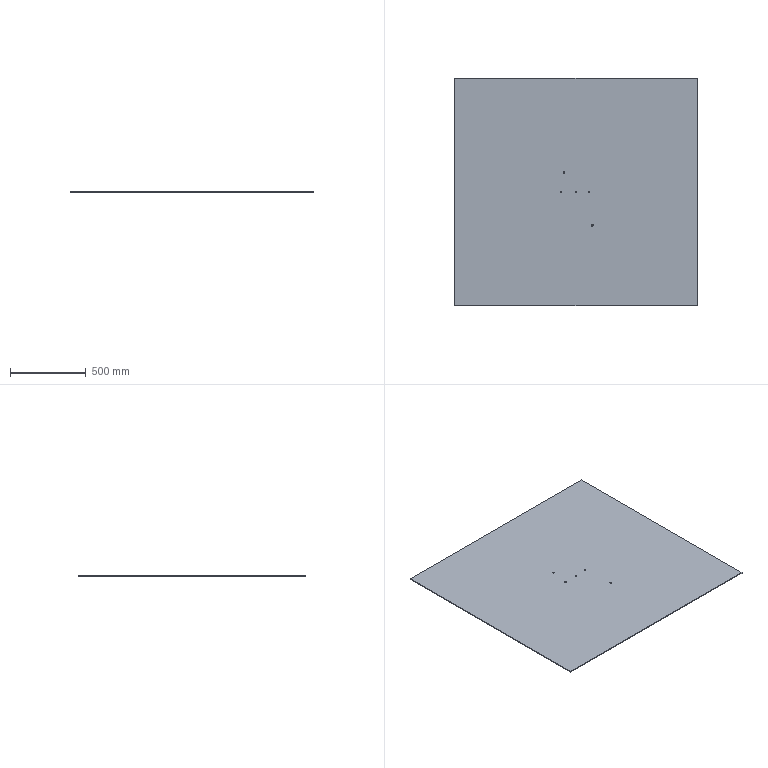Part | SolidWorks | features Extrusion 1 | 1 solid | 16 faces | box 1600 x 1500 x 5 mm | volume 11997688 mm3 | cylinder 10 | plane 6 | commonest cylinder face diameters 10 x6 10.014 x2 13.731 x2
STEP:
#1=CARTESIAN_POINT('',(-84.757,130.,5.));
#2=VERTEX_POINT('',#1);
#3=CARTESIAN_POINT('',(-74.743,130.,5.));
#4=VERTEX_POINT('',#3);
#5=CARTESIAN_POINT('',(-79.75,130.,5.));
#6=DIRECTION('',(0.,0.,1.));
#7=DIRECTION('',(1.,0.,0.));
#8=AXIS2_PLACEMENT_3D('',#5,#6,#7);
#9=CIRCLE('',#8,5.007);
#10=EDGE_CURVE('',#2,#4,#9,.T.);
#11=ORIENTED_EDGE('',*,*,#10,.T.);
#12=CARTESIAN_POINT('',(-74.743,130.,0.));
#13=VERTEX_POINT('',#12);
#14=CARTESIAN_POINT('',(-74.743,130.,5.));
#15=DIRECTION('',(0.,0.,-1.));
#16=VECTOR('',#15,1000.);
#17=LINE('',#14,#16);
#18=EDGE_CURVE('',#4,#13,#17,.T.);
#19=ORIENTED_EDGE('',*,*,#18,.T.);
#20=CARTESIAN_POINT('',(-84.757,130.,0.));
#21=VERTEX_POINT('',#20);
#22=CARTESIAN_POINT('',(-79.75,130.,0.));
#23=DIRECTION('',(0.,0.,1.));
#24=DIRECTION('',(1.,0.,0.));
#25=AXIS2_PLACEMENT_3D('',#22,#23,#24);
#26=CIRCLE('',#25,5.007);
#27=EDGE_CURVE('',#21,#13,#26,.T.);
#28=ORIENTED_EDGE('',*,*,#27,.F.);
#29=CARTESIAN_POINT('',(-84.757,130.,5.));
#30=DIRECTION('',(0.,0.,-1.));
#31=VECTOR('',#30,1000.);
#32=LINE('',#29,#31);
#33=EDGE_CURVE('',#2,#21,#32,.T.);
#34=ORIENTED_EDGE('',*,*,#33,.F.);
#35=EDGE_LOOP('',(#11,#19,#28,#34));
#36=FACE_OUTER_BOUND('',#35,.T.);
#37=CARTESIAN_POINT('',(-79.75,130.,5.));
#38=DIRECTION('',(0.,0.,-1.));
#39=DIRECTION('',(-1.,0.,0.));
#40=AXIS2_PLACEMENT_3D('',#37,#38,#39);
#41=CYLINDRICAL_SURFACE('',#40,5.007);
#42=ADVANCED_FACE('',(#36),#41,.F.);
#43=CARTESIAN_POINT('',(99.385,-219.089,5.));
#44=VERTEX_POINT('',#43);
#45=CARTESIAN_POINT('',(113.115,-219.089,5.));
#46=VERTEX_POINT('',#45);
#47=CARTESIAN_POINT('',(106.25,-219.089,5.));
#48=DIRECTION('',(0.,0.,1.));
#49=DIRECTION('',(1.,0.,0.));
#50=AXIS2_PLACEMENT_3D('',#47,#48,#49);
#51=CIRCLE('',#50,6.865);
#52=EDGE_CURVE('',#44,#46,#51,.T.);
#53=ORIENTED_EDGE('',*,*,#52,.T.);
#54=CARTESIAN_POINT('',(113.115,-219.089,0.));
#55=VERTEX_POINT('',#54);
#56=CARTESIAN_POINT('',(113.115,-219.089,5.));
#57=DIRECTION('',(0.,0.,-1.));
#58=VECTOR('',#57,1000.);
#59=LINE('',#56,#58);
#60=EDGE_CURVE('',#46,#55,#59,.T.);
#61=ORIENTED_EDGE('',*,*,#60,.T.);
#62=CARTESIAN_POINT('',(99.385,-219.089,0.));
#63=VERTEX_POINT('',#62);
#64=CARTESIAN_POINT('',(106.25,-219.089,0.));
#65=DIRECTION('',(0.,0.,1.));
#66=DIRECTION('',(1.,0.,0.));
#67=AXIS2_PLACEMENT_3D('',#64,#65,#66);
#68=CIRCLE('',#67,6.865);
#69=EDGE_CURVE('',#63,#55,#68,.T.);
#70=ORIENTED_EDGE('',*,*,#69,.F.);
#71=CARTESIAN_POINT('',(99.385,-219.089,5.));
#72=DIRECTION('',(0.,0.,-1.));
#73=VECTOR('',#72,1000.);
#74=LINE('',#71,#73);
#75=EDGE_CURVE('',#44,#63,#74,.T.);
#76=ORIENTED_EDGE('',*,*,#75,.F.);
#77=EDGE_LOOP('',(#53,#61,#70,#76));
#78=FACE_OUTER_BOUND('',#77,.T.);
#79=CARTESIAN_POINT('',(106.25,-219.089,5.));
#80=DIRECTION('',(0.,0.,-1.));
#81=DIRECTION('',(-1.,0.,0.));
#82=AXIS2_PLACEMENT_3D('',#79,#80,#81);
#83=CYLINDRICAL_SURFACE('',#82,6.865);
#84=ADVANCED_FACE('',(#78),#83,.F.);
#85=CARTESIAN_POINT('',(81.25,0.,5.));
#86=VERTEX_POINT('',#85);
#87=CARTESIAN_POINT('',(91.25,0.,5.));
#88=VERTEX_POINT('',#87);
#89=CARTESIAN_POINT('',(86.25,0.,5.));
#90=DIRECTION('',(0.,0.,1.));
#91=DIRECTION('',(1.,0.,0.));
#92=AXIS2_PLACEMENT_3D('',#89,#90,#91);
#93=CIRCLE('',#92,5.);
#94=EDGE_CURVE('',#86,#88,#93,.T.);
#95=ORIENTED_EDGE('',*,*,#94,.T.);
#96=CARTESIAN_POINT('',(91.25,0.,0.));
#97=VERTEX_POINT('',#96);
#98=CARTESIAN_POINT('',(91.25,0.,5.));
#99=DIRECTION('',(0.,0.,-1.));
#100=VECTOR('',#99,1000.);
#101=LINE('',#98,#100);
#102=EDGE_CURVE('',#88,#97,#101,.T.);
#103=ORIENTED_EDGE('',*,*,#102,.T.);
#104=CARTESIAN_POINT('',(81.25,0.,0.));
#105=VERTEX_POINT('',#104);
#106=CARTESIAN_POINT('',(86.25,0.,0.));
#107=DIRECTION('',(0.,0.,1.));
#108=DIRECTION('',(1.,0.,0.));
#109=AXIS2_PLACEMENT_3D('',#106,#107,#108);
#110=CIRCLE('',#109,5.);
#111=EDGE_CURVE('',#105,#97,#110,.T.);
#112=ORIENTED_EDGE('',*,*,#111,.F.);
#113=CARTESIAN_POINT('',(81.25,0.,5.));
#114=DIRECTION('',(0.,0.,-1.));
#115=VECTOR('',#114,1000.);
#116=LINE('',#113,#115);
#117=EDGE_CURVE('',#86,#105,#116,.T.);
#118=ORIENTED_EDGE('',*,*,#117,.F.);
#119=EDGE_LOOP('',(#95,#103,#112,#118));
#120=FACE_OUTER_BOUND('',#119,.T.);
#121=CARTESIAN_POINT('',(86.25,0.,5.));
#122=DIRECTION('',(0.,0.,-1.));
#123=DIRECTION('',(-1.,0.,0.));
#124=AXIS2_PLACEMENT_3D('',#121,#122,#123);
#125=CYLINDRICAL_SURFACE('',#124,5.);
#126=ADVANCED_FACE('',(#120),#125,.F.);
#127=CARTESIAN_POINT('',(-104.75,0.,5.));
#128=VERTEX_POINT('',#127);
#129=CARTESIAN_POINT('',(-94.75,0.,5.));
#130=VERTEX_POINT('',#129);
#131=CARTESIAN_POINT('',(-99.75,0.,5.));
#132=DIRECTION('',(0.,0.,1.));
#133=DIRECTION('',(1.,0.,0.));
#134=AXIS2_PLACEMENT_3D('',#131,#132,#133);
#135=CIRCLE('',#134,5.);
#136=EDGE_CURVE('',#128,#130,#135,.T.);
#137=ORIENTED_EDGE('',*,*,#136,.T.);
#138=CARTESIAN_POINT('',(-94.75,0.,0.));
#139=VERTEX_POINT('',#138);
#140=CARTESIAN_POINT('',(-94.75,0.,5.));
#141=DIRECTION('',(0.,0.,-1.));
#142=VECTOR('',#141,1000.);
#143=LINE('',#140,#142);
#144=EDGE_CURVE('',#130,#139,#143,.T.);
#145=ORIENTED_EDGE('',*,*,#144,.T.);
#146=CARTESIAN_POINT('',(-104.75,0.,0.));
#147=VERTEX_POINT('',#146);
#148=CARTESIAN_POINT('',(-99.75,0.,0.));
#149=DIRECTION('',(0.,0.,1.));
#150=DIRECTION('',(1.,0.,0.));
#151=AXIS2_PLACEMENT_3D('',#148,#149,#150);
#152=CIRCLE('',#151,5.);
#153=EDGE_CURVE('',#147,#139,#152,.T.);
#154=ORIENTED_EDGE('',*,*,#153,.F.);
#155=CARTESIAN_POINT('',(-104.75,0.,5.));
#156=DIRECTION('',(0.,0.,-1.));
#157=VECTOR('',#156,1000.);
#158=LINE('',#155,#157);
#159=EDGE_CURVE('',#128,#147,#158,.T.);
#160=ORIENTED_EDGE('',*,*,#159,.F.);
#161=EDGE_LOOP('',(#137,#145,#154,#160));
#162=FACE_OUTER_BOUND('',#161,.T.);
#163=CARTESIAN_POINT('',(-99.75,0.,5.));
#164=DIRECTION('',(0.,0.,-1.));
#165=DIRECTION('',(-1.,0.,0.));
#166=AXIS2_PLACEMENT_3D('',#163,#164,#165);
#167=CYLINDRICAL_SURFACE('',#166,5.);
#168=ADVANCED_FACE('',(#162),#167,.F.);
#169=CARTESIAN_POINT('',(-5.,0.,5.));
#170=VERTEX_POINT('',#169);
#171=CARTESIAN_POINT('',(5.,0.,5.));
#172=VERTEX_POINT('',#171);
#173=CARTESIAN_POINT('',(0.,0.,5.));
#174=DIRECTION('',(0.,0.,1.));
#175=DIRECTION('',(1.,0.,0.));
#176=AXIS2_PLACEMENT_3D('',#173,#174,#175);
#177=CIRCLE('',#176,5.);
#178=EDGE_CURVE('',#170,#172,#177,.T.);
#179=ORIENTED_EDGE('',*,*,#178,.T.);
#180=CARTESIAN_POINT('',(5.,0.,0.));
#181=VERTEX_POINT('',#180);
#182=CARTESIAN_POINT('',(5.,0.,5.));
#183=DIRECTION('',(0.,0.,-1.));
#184=VECTOR('',#183,1000.);
#185=LINE('',#182,#184);
#186=EDGE_CURVE('',#172,#181,#185,.T.);
#187=ORIENTED_EDGE('',*,*,#186,.T.);
#188=CARTESIAN_POINT('',(-5.,0.,0.));
#189=VERTEX_POINT('',#188);
#190=CARTESIAN_POINT('',(0.,0.,0.));
#191=DIRECTION('',(0.,0.,1.));
#192=DIRECTION('',(1.,0.,0.));
#193=AXIS2_PLACEMENT_3D('',#190,#191,#192);
#194=CIRCLE('',#193,5.);
#195=EDGE_CURVE('',#189,#181,#194,.T.);
#196=ORIENTED_EDGE('',*,*,#195,.F.);
#197=CARTESIAN_POINT('',(-5.,0.,5.));
#198=DIRECTION('',(0.,0.,-1.));
#199=VECTOR('',#198,1000.);
#200=LINE('',#197,#199);
#201=EDGE_CURVE('',#170,#189,#200,.T.);
#202=ORIENTED_EDGE('',*,*,#201,.F.);
#203=EDGE_LOOP('',(#179,#187,#196,#202));
#204=FACE_OUTER_BOUND('',#203,.T.);
#205=CARTESIAN_POINT('',(0.,0.,5.));
#206=DIRECTION('',(0.,0.,-1.));
#207=DIRECTION('',(-1.,0.,0.));
#208=AXIS2_PLACEMENT_3D('',#205,#206,#207);
#209=CYLINDRICAL_SURFACE('',#208,5.);
#210=ADVANCED_FACE('',(#204),#209,.F.);
#211=ORIENTED_EDGE('',*,*,#52,.F.);
#212=CARTESIAN_POINT('',(106.25,-219.089,5.));
#213=DIRECTION('',(0.,0.,1.));
#214=DIRECTION('',(1.,0.,0.));
#215=AXIS2_PLACEMENT_3D('',#212,#213,#214);
#216=CIRCLE('',#215,6.865);
#217=EDGE_CURVE('',#46,#44,#216,.T.);
#218=ORIENTED_EDGE('',*,*,#217,.F.);
#219=EDGE_LOOP('',(#211,#218));
#220=FACE_BOUND('',#219,.T.);
#221=ORIENTED_EDGE('',*,*,#136,.F.);
#222=CARTESIAN_POINT('',(-99.75,0.,5.));
#223=DIRECTION('',(0.,0.,1.));
#224=DIRECTION('',(1.,0.,0.));
#225=AXIS2_PLACEMENT_3D('',#222,#223,#224);
#226=CIRCLE('',#225,5.);
#227=EDGE_CURVE('',#130,#128,#226,.T.);
#228=ORIENTED_EDGE('',*,*,#227,.F.);
#229=EDGE_LOOP('',(#221,#228));
#230=FACE_BOUND('',#229,.T.);
#231=CARTESIAN_POINT('',(800.,-750.,5.));
#232=VERTEX_POINT('',#231);
#233=CARTESIAN_POINT('',(800.,750.,5.));
#234=VERTEX_POINT('',#233);
#235=CARTESIAN_POINT('',(800.,750.,5.));
#236=DIRECTION('',(0.,1.,0.));
#237=VECTOR('',#236,1000.);
#238=LINE('',#235,#237);
#239=EDGE_CURVE('',#232,#234,#238,.T.);
#240=ORIENTED_EDGE('',*,*,#239,.T.);
#241=CARTESIAN_POINT('',(-800.,750.,5.));
#242=VERTEX_POINT('',#241);
#243=CARTESIAN_POINT('',(-800.,750.,5.));
#244=DIRECTION('',(-1.,0.,0.));
#245=VECTOR('',#244,1000.);
#246=LINE('',#243,#245);
#247=EDGE_CURVE('',#234,#242,#246,.T.);
#248=ORIENTED_EDGE('',*,*,#247,.T.);
#249=CARTESIAN_POINT('',(-800.,-750.,5.));
#250=VERTEX_POINT('',#249);
#251=CARTESIAN_POINT('',(-800.,750.,5.));
#252=DIRECTION('',(0.,-1.,0.));
#253=VECTOR('',#252,1000.);
#254=LINE('',#251,#253);
#255=EDGE_CURVE('',#242,#250,#254,.T.);
#256=ORIENTED_EDGE('',*,*,#255,.T.);
#257=CARTESIAN_POINT('',(-800.,-750.,5.));
#258=DIRECTION('',(1.,0.,0.));
#259=VECTOR('',#258,1000.);
#260=LINE('',#257,#259);
#261=EDGE_CURVE('',#250,#232,#260,.T.);
#262=ORIENTED_EDGE('',*,*,#261,.T.);
#263=EDGE_LOOP('',(#240,#248,#256,#262));
#264=FACE_OUTER_BOUND('',#263,.T.);
#265=ORIENTED_EDGE('',*,*,#178,.F.);
#266=CARTESIAN_POINT('',(0.,0.,5.));
#267=DIRECTION('',(0.,0.,1.));
#268=DIRECTION('',(1.,0.,0.));
#269=AXIS2_PLACEMENT_3D('',#266,#267,#268);
#270=CIRCLE('',#269,5.);
#271=EDGE_CURVE('',#172,#170,#270,.T.);
#272=ORIENTED_EDGE('',*,*,#271,.F.);
#273=EDGE_LOOP('',(#265,#272));
#274=FACE_BOUND('',#273,.T.);
#275=ORIENTED_EDGE('',*,*,#94,.F.);
#276=CARTESIAN_POINT('',(86.25,0.,5.));
#277=DIRECTION('',(0.,0.,1.));
#278=DIRECTION('',(1.,0.,0.));
#279=AXIS2_PLACEMENT_3D('',#276,#277,#278);
#280=CIRCLE('',#279,5.);
#281=EDGE_CURVE('',#88,#86,#280,.T.);
#282=ORIENTED_EDGE('',*,*,#281,.F.);
#283=EDGE_LOOP('',(#275,#282));
#284=FACE_BOUND('',#283,.T.);
#285=ORIENTED_EDGE('',*,*,#10,.F.);
#286=CARTESIAN_POINT('',(-79.75,130.,5.));
#287=DIRECTION('',(0.,0.,1.));
#288=DIRECTION('',(1.,0.,0.));
#289=AXIS2_PLACEMENT_3D('',#286,#287,#288);
#290=CIRCLE('',#289,5.007);
#291=EDGE_CURVE('',#4,#2,#290,.T.);
#292=ORIENTED_EDGE('',*,*,#291,.F.);
#293=EDGE_LOOP('',(#285,#292));
#294=FACE_BOUND('',#293,.T.);
#295=CARTESIAN_POINT('',(0.,0.,5.));
#296=DIRECTION('',(0.,0.,1.));
#297=DIRECTION('',(1.,0.,0.));
#298=AXIS2_PLACEMENT_3D('',#295,#296,#297);
#299=PLANE('',#298);
#300=ADVANCED_FACE('',(#220,#230,#264,#274,#284,#294),#299,.T.);
#301=CARTESIAN_POINT('',(800.,-750.,0.));
#302=VERTEX_POINT('',#301);
#303=CARTESIAN_POINT('',(800.,750.,0.));
#304=VERTEX_POINT('',#303);
#305=CARTESIAN_POINT('',(800.,750.,0.));
#306=DIRECTION('',(0.,1.,0.));
#307=VECTOR('',#306,1000.);
#308=LINE('',#305,#307);
#309=EDGE_CURVE('',#302,#304,#308,.T.);
#310=ORIENTED_EDGE('',*,*,#309,.F.);
#311=CARTESIAN_POINT('',(-800.,-750.,0.));
#312=VERTEX_POINT('',#311);
#313=CARTESIAN_POINT('',(-800.,-750.,0.));
#314=DIRECTION('',(1.,0.,0.));
#315=VECTOR('',#314,1000.);
#316=LINE('',#313,#315);
#317=EDGE_CURVE('',#312,#302,#316,.T.);
#318=ORIENTED_EDGE('',*,*,#317,.F.);
#319=CARTESIAN_POINT('',(-800.,750.,0.));
#320=VERTEX_POINT('',#319);
#321=CARTESIAN_POINT('',(-800.,750.,0.));
#322=DIRECTION('',(0.,-1.,0.));
#323=VECTOR('',#322,1000.);
#324=LINE('',#321,#323);
#325=EDGE_CURVE('',#320,#312,#324,.T.);
#326=ORIENTED_EDGE('',*,*,#325,.F.);
#327=CARTESIAN_POINT('',(-800.,750.,0.));
#328=DIRECTION('',(-1.,0.,0.));
#329=VECTOR('',#328,1000.);
#330=LINE('',#327,#329);
#331=EDGE_CURVE('',#304,#320,#330,.T.);
#332=ORIENTED_EDGE('',*,*,#331,.F.);
#333=EDGE_LOOP('',(#310,#318,#326,#332));
#334=FACE_OUTER_BOUND('',#333,.T.);
#335=ORIENTED_EDGE('',*,*,#195,.T.);
#336=CARTESIAN_POINT('',(0.,0.,0.));
#337=DIRECTION('',(0.,0.,1.));
#338=DIRECTION('',(1.,0.,0.));
#339=AXIS2_PLACEMENT_3D('',#336,#337,#338);
#340=CIRCLE('',#339,5.);
#341=EDGE_CURVE('',#181,#189,#340,.T.);
#342=ORIENTED_EDGE('',*,*,#341,.T.);
#343=EDGE_LOOP('',(#335,#342));
#344=FACE_BOUND('',#343,.T.);
#345=ORIENTED_EDGE('',*,*,#153,.T.);
#346=CARTESIAN_POINT('',(-99.75,0.,0.));
#347=DIRECTION('',(0.,0.,1.));
#348=DIRECTION('',(1.,0.,0.));
#349=AXIS2_PLACEMENT_3D('',#346,#347,#348);
#350=CIRCLE('',#349,5.);
#351=EDGE_CURVE('',#139,#147,#350,.T.);
#352=ORIENTED_EDGE('',*,*,#351,.T.);
#353=EDGE_LOOP('',(#345,#352));
#354=FACE_BOUND('',#353,.T.);
#355=ORIENTED_EDGE('',*,*,#111,.T.);
#356=CARTESIAN_POINT('',(86.25,0.,0.));
#357=DIRECTION('',(0.,0.,1.));
#358=DIRECTION('',(1.,0.,0.));
#359=AXIS2_PLACEMENT_3D('',#356,#357,#358);
#360=CIRCLE('',#359,5.);
#361=EDGE_CURVE('',#97,#105,#360,.T.);
#362=ORIENTED_EDGE('',*,*,#361,.T.);
#363=EDGE_LOOP('',(#355,#362));
#364=FACE_BOUND('',#363,.T.);
#365=ORIENTED_EDGE('',*,*,#69,.T.);
#366=CARTESIAN_POINT('',(106.25,-219.089,0.));
#367=DIRECTION('',(0.,0.,1.));
#368=DIRECTION('',(1.,0.,0.));
#369=AXIS2_PLACEMENT_3D('',#366,#367,#368);
#370=CIRCLE('',#369,6.865);
#371=EDGE_CURVE('',#55,#63,#370,.T.);
#372=ORIENTED_EDGE('',*,*,#371,.T.);
#373=EDGE_LOOP('',(#365,#372));
#374=FACE_BOUND('',#373,.T.);
#375=ORIENTED_EDGE('',*,*,#27,.T.);
#376=CARTESIAN_POINT('',(-79.75,130.,0.));
#377=DIRECTION('',(0.,0.,1.));
#378=DIRECTION('',(1.,0.,0.));
#379=AXIS2_PLACEMENT_3D('',#376,#377,#378);
#380=CIRCLE('',#379,5.007);
#381=EDGE_CURVE('',#13,#21,#380,.T.);
#382=ORIENTED_EDGE('',*,*,#381,.T.);
#383=EDGE_LOOP('',(#375,#382));
#384=FACE_BOUND('',#383,.T.);
#385=CARTESIAN_POINT('',(0.,0.,0.));
#386=DIRECTION('',(0.,0.,1.));
#387=DIRECTION('',(1.,0.,0.));
#388=AXIS2_PLACEMENT_3D('',#385,#386,#387);
#389=PLANE('',#388);
#390=ADVANCED_FACE('',(#334,#344,#354,#364,#374,#384),#389,.F.);
#391=ORIENTED_EDGE('',*,*,#309,.T.);
#392=CARTESIAN_POINT('',(800.,750.,5.));
#393=DIRECTION('',(0.,0.,-1.));
#394=VECTOR('',#393,1000.);
#395=LINE('',#392,#394);
#396=EDGE_CURVE('',#234,#304,#395,.T.);
#397=ORIENTED_EDGE('',*,*,#396,.F.);
#398=ORIENTED_EDGE('',*,*,#239,.F.);
#399=CARTESIAN_POINT('',(800.,-750.,5.));
#400=DIRECTION('',(0.,0.,-1.));
#401=VECTOR('',#400,1000.);
#402=LINE('',#399,#401);
#403=EDGE_CURVE('',#232,#302,#402,.T.);
#404=ORIENTED_EDGE('',*,*,#403,.T.);
#405=EDGE_LOOP('',(#391,#397,#398,#404));
#406=FACE_OUTER_BOUND('',#405,.T.);
#407=CARTESIAN_POINT('',(800.,750.,5.));
#408=DIRECTION('',(-1.,0.,0.));
#409=DIRECTION('',(0.,0.,1.));
#410=AXIS2_PLACEMENT_3D('',#407,#408,#409);
#411=PLANE('',#410);
#412=ADVANCED_FACE('',(#406),#411,.F.);
#413=ORIENTED_EDGE('',*,*,#331,.T.);
#414=CARTESIAN_POINT('',(-800.,750.,5.));
#415=DIRECTION('',(0.,0.,-1.));
#416=VECTOR('',#415,1000.);
#417=LINE('',#414,#416);
#418=EDGE_CURVE('',#242,#320,#417,.T.);
#419=ORIENTED_EDGE('',*,*,#418,.F.);
#420=ORIENTED_EDGE('',*,*,#247,.F.);
#421=ORIENTED_EDGE('',*,*,#396,.T.);
#422=EDGE_LOOP('',(#413,#419,#420,#421));
#423=FACE_OUTER_BOUND('',#422,.T.);
#424=CARTESIAN_POINT('',(-800.,750.,5.));
#425=DIRECTION('',(0.,-1.,0.));
#426=DIRECTION('',(0.,0.,-1.));
#427=AXIS2_PLACEMENT_3D('',#424,#425,#426);
#428=PLANE('',#427);
#429=ADVANCED_FACE('',(#423),#428,.F.);
#430=ORIENTED_EDGE('',*,*,#325,.T.);
#431=CARTESIAN_POINT('',(-800.,-750.,5.));
#432=DIRECTION('',(0.,0.,-1.));
#433=VECTOR('',#432,1000.);
#434=LINE('',#431,#433);
#435=EDGE_CURVE('',#250,#312,#434,.T.);
#436=ORIENTED_EDGE('',*,*,#435,.F.);
#437=ORIENTED_EDGE('',*,*,#255,.F.);
#438=ORIENTED_EDGE('',*,*,#418,.T.);
#439=EDGE_LOOP('',(#430,#436,#437,#438));
#440=FACE_OUTER_BOUND('',#439,.T.);
#441=CARTESIAN_POINT('',(-800.,750.,5.));
#442=DIRECTION('',(1.,0.,0.));
#443=DIRECTION('',(0.,1.,0.));
#444=AXIS2_PLACEMENT_3D('',#441,#442,#443);
#445=PLANE('',#444);
#446=ADVANCED_FACE('',(#440),#445,.F.);
#447=ORIENTED_EDGE('',*,*,#317,.T.);
#448=ORIENTED_EDGE('',*,*,#403,.F.);
#449=ORIENTED_EDGE('',*,*,#261,.F.);
#450=ORIENTED_EDGE('',*,*,#435,.T.);
#451=EDGE_LOOP('',(#447,#448,#449,#450));
#452=FACE_OUTER_BOUND('',#451,.T.);
#453=CARTESIAN_POINT('',(-800.,-750.,5.));
#454=DIRECTION('',(0.,1.,0.));
#455=DIRECTION('',(-1.,0.,0.));
#456=AXIS2_PLACEMENT_3D('',#453,#454,#455);
#457=PLANE('',#456);
#458=ADVANCED_FACE('',(#452),#457,.F.);
#459=ORIENTED_EDGE('',*,*,#186,.F.);
#460=ORIENTED_EDGE('',*,*,#271,.T.);
#461=ORIENTED_EDGE('',*,*,#201,.T.);
#462=ORIENTED_EDGE('',*,*,#341,.F.);
#463=EDGE_LOOP('',(#459,#460,#461,#462));
#464=FACE_OUTER_BOUND('',#463,.T.);
#465=CARTESIAN_POINT('',(0.,0.,5.));
#466=DIRECTION('',(0.,0.,-1.));
#467=DIRECTION('',(-1.,0.,0.));
#468=AXIS2_PLACEMENT_3D('',#465,#466,#467);
#469=CYLINDRICAL_SURFACE('',#468,5.);
#470=ADVANCED_FACE('',(#464),#469,.F.);
#471=ORIENTED_EDGE('',*,*,#144,.F.);
#472=ORIENTED_EDGE('',*,*,#227,.T.);
#473=ORIENTED_EDGE('',*,*,#159,.T.);
#474=ORIENTED_EDGE('',*,*,#351,.F.);
#475=EDGE_LOOP('',(#471,#472,#473,#474));
#476=FACE_OUTER_BOUND('',#475,.T.);
#477=CARTESIAN_POINT('',(-99.75,0.,5.));
#478=DIRECTION('',(0.,0.,-1.));
#479=DIRECTION('',(-1.,0.,0.));
#480=AXIS2_PLACEMENT_3D('',#477,#478,#479);
#481=CYLINDRICAL_SURFACE('',#480,5.);
#482=ADVANCED_FACE('',(#476),#481,.F.);
#483=ORIENTED_EDGE('',*,*,#102,.F.);
#484=ORIENTED_EDGE('',*,*,#281,.T.);
#485=ORIENTED_EDGE('',*,*,#117,.T.);
#486=ORIENTED_EDGE('',*,*,#361,.F.);
#487=EDGE_LOOP('',(#483,#484,#485,#486));
#488=FACE_OUTER_BOUND('',#487,.T.);
#489=CARTESIAN_POINT('',(86.25,0.,5.));
#490=DIRECTION('',(0.,0.,-1.));
#491=DIRECTION('',(-1.,0.,0.));
#492=AXIS2_PLACEMENT_3D('',#489,#490,#491);
#493=CYLINDRICAL_SURFACE('',#492,5.);
#494=ADVANCED_FACE('',(#488),#493,.F.);
#495=ORIENTED_EDGE('',*,*,#60,.F.);
#496=ORIENTED_EDGE('',*,*,#217,.T.);
#497=ORIENTED_EDGE('',*,*,#75,.T.);
#498=ORIENTED_EDGE('',*,*,#371,.F.);
#499=EDGE_LOOP('',(#495,#496,#497,#498));
#500=FACE_OUTER_BOUND('',#499,.T.);
#501=CARTESIAN_POINT('',(106.25,-219.089,5.));
#502=DIRECTION('',(0.,0.,-1.));
#503=DIRECTION('',(-1.,0.,0.));
#504=AXIS2_PLACEMENT_3D('',#501,#502,#503);
#505=CYLINDRICAL_SURFACE('',#504,6.865);
#506=ADVANCED_FACE('',(#500),#505,.F.);
#507=ORIENTED_EDGE('',*,*,#18,.F.);
#508=ORIENTED_EDGE('',*,*,#291,.T.);
#509=ORIENTED_EDGE('',*,*,#33,.T.);
#510=ORIENTED_EDGE('',*,*,#381,.F.);
#511=EDGE_LOOP('',(#507,#508,#509,#510));
#512=FACE_OUTER_BOUND('',#511,.T.);
#513=CARTESIAN_POINT('',(-79.75,130.,5.));
#514=DIRECTION('',(0.,0.,-1.));
#515=DIRECTION('',(-1.,0.,0.));
#516=AXIS2_PLACEMENT_3D('',#513,#514,#515);
#517=CYLINDRICAL_SURFACE('',#516,5.007);
#518=ADVANCED_FACE('',(#512),#517,.F.);
#519=CLOSED_SHELL('',(#42,#84,#126,#168,#210,#300,#390,#412,#429,#446,#458,#470,#482,#494,#506,#518));
#520=MANIFOLD_SOLID_BREP('',#519);
#521=CARTESIAN_POINT('',(0.,0.,0.));
#522=DIRECTION('',(0.,0.,1.));
#523=DIRECTION('',(1.,0.,0.));
#524=AXIS2_PLACEMENT_3D('',#521,#522,#523);
#525=(LENGTH_UNIT()NAMED_UNIT(*)SI_UNIT(.MILLI.,.METRE.));
#526=UNCERTAINTY_MEASURE_WITH_UNIT(LENGTH_MEASURE(0.00001),#525,'','');
#527=(NAMED_UNIT(*)PLANE_ANGLE_UNIT()SI_UNIT($,.RADIAN.));
#528=(NAMED_UNIT(*)SI_UNIT($,.STERADIAN.)SOLID_ANGLE_UNIT());
#529=(GEOMETRIC_REPRESENTATION_CONTEXT(3)GLOBAL_UNCERTAINTY_ASSIGNED_CONTEXT((#526))GLOBAL_UNIT_ASSIGNED_CONTEXT((#525,#527,#528))REPRESENTATION_CONTEXT('',''));
#530=ADVANCED_BREP_SHAPE_REPRESENTATION('',(#520,#524),#529);